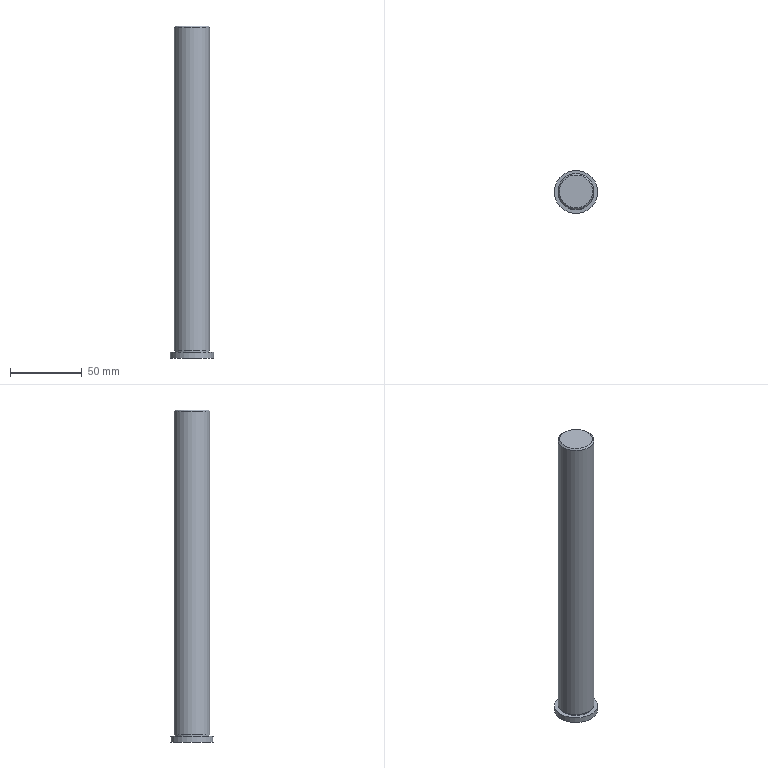Part | STEP file | 1_id634_xmt_txt | 1 solid | 8 faces | box 30 x 30 x 231 mm | volume 114179 mm3 | plane 4 | cylinder 3 | cone 1 | commonest cylinder face diameters 24 x1 25 x1 30 x1
STEP:
#1=CARTESIAN_POINT('',(-84.,-130.,-214.));
#2=VERTEX_POINT('',#1);
#3=CARTESIAN_POINT('',(-99.,-130.,-214.));
#4=DIRECTION('',(0.,0.,-1.));
#5=DIRECTION('',(1.,0.,0.));
#6=AXIS2_PLACEMENT_3D('',#3,#4,#5);
#7=CIRCLE('',#6,15.);
#8=EDGE_CURVE('',#2,#2,#7,.T.);
#9=ORIENTED_EDGE('',*,*,#8,.F.);
#10=EDGE_LOOP('',(#9));
#11=FACE_BOUND('',#10,.T.);
#12=CARTESIAN_POINT('',(-84.,-130.,-210.));
#13=VERTEX_POINT('',#12);
#14=CARTESIAN_POINT('',(-99.,-130.,-210.));
#15=DIRECTION('',(0.,0.,1.));
#16=DIRECTION('',(1.,0.,0.));
#17=AXIS2_PLACEMENT_3D('',#14,#15,#16);
#18=CIRCLE('',#17,15.);
#19=EDGE_CURVE('',#13,#13,#18,.T.);
#20=ORIENTED_EDGE('',*,*,#19,.F.);
#21=EDGE_LOOP('',(#20));
#22=FACE_BOUND('',#21,.T.);
#23=CARTESIAN_POINT('',(-99.,-130.,-212.));
#24=DIRECTION('',(0.,0.,1.));
#25=DIRECTION('',(-1.,0.,0.));
#26=AXIS2_PLACEMENT_3D('',#23,#24,#25);
#27=CYLINDRICAL_SURFACE('',#26,15.);
#28=ADVANCED_FACE('',(#11,#22),#27,.T.);
#29=CARTESIAN_POINT('',(-111.,-130.,-209.));
#30=VERTEX_POINT('',#29);
#31=CARTESIAN_POINT('',(-99.,-130.,-209.));
#32=DIRECTION('',(0.,0.,1.));
#33=DIRECTION('',(-1.,0.,0.));
#34=AXIS2_PLACEMENT_3D('',#31,#32,#33);
#35=CIRCLE('',#34,12.);
#36=EDGE_CURVE('',#30,#30,#35,.T.);
#37=ORIENTED_EDGE('',*,*,#36,.F.);
#38=EDGE_LOOP('',(#37));
#39=FACE_BOUND('',#38,.T.);
#40=CARTESIAN_POINT('',(-111.,-130.,-210.));
#41=VERTEX_POINT('',#40);
#42=CARTESIAN_POINT('',(-99.,-130.,-210.));
#43=DIRECTION('',(0.,0.,1.));
#44=DIRECTION('',(-1.,0.,0.));
#45=AXIS2_PLACEMENT_3D('',#42,#43,#44);
#46=CIRCLE('',#45,12.);
#47=EDGE_CURVE('',#41,#41,#46,.T.);
#48=ORIENTED_EDGE('',*,*,#47,.T.);
#49=EDGE_LOOP('',(#48));
#50=FACE_BOUND('',#49,.T.);
#51=CARTESIAN_POINT('',(-99.,-130.,-209.5));
#52=DIRECTION('',(0.,0.,1.));
#53=DIRECTION('',(1.,0.,0.));
#54=AXIS2_PLACEMENT_3D('',#51,#52,#53);
#55=CYLINDRICAL_SURFACE('',#54,12.);
#56=ADVANCED_FACE('',(#39,#50),#55,.T.);
#57=CARTESIAN_POINT('',(-86.5,-130.,-209.));
#58=VERTEX_POINT('',#57);
#59=CARTESIAN_POINT('',(-99.,-130.,-209.));
#60=DIRECTION('',(0.,0.,1.));
#61=DIRECTION('',(1.,0.,0.));
#62=AXIS2_PLACEMENT_3D('',#59,#60,#61);
#63=CIRCLE('',#62,12.5);
#64=EDGE_CURVE('',#58,#58,#63,.T.);
#65=ORIENTED_EDGE('',*,*,#64,.T.);
#66=EDGE_LOOP('',(#65));
#67=FACE_BOUND('',#66,.T.);
#68=CARTESIAN_POINT('',(-111.5,-130.,16.));
#69=VERTEX_POINT('',#68);
#70=CARTESIAN_POINT('',(-99.,-130.,16.));
#71=DIRECTION('',(0.,0.,1.));
#72=DIRECTION('',(-1.,0.,0.));
#73=AXIS2_PLACEMENT_3D('',#70,#71,#72);
#74=CIRCLE('',#73,12.5);
#75=EDGE_CURVE('',#69,#69,#74,.T.);
#76=ORIENTED_EDGE('',*,*,#75,.F.);
#77=EDGE_LOOP('',(#76));
#78=FACE_BOUND('',#77,.T.);
#79=CARTESIAN_POINT('',(-99.,-130.,-96.5));
#80=DIRECTION('',(0.,0.,1.));
#81=DIRECTION('',(-1.,0.,0.));
#82=AXIS2_PLACEMENT_3D('',#79,#80,#81);
#83=CYLINDRICAL_SURFACE('',#82,12.5);
#84=ADVANCED_FACE('',(#67,#78),#83,.T.);
#85=ORIENTED_EDGE('',*,*,#75,.T.);
#86=EDGE_LOOP('',(#85));
#87=FACE_BOUND('',#86,.T.);
#88=CARTESIAN_POINT('',(-110.5,-130.,17.));
#89=VERTEX_POINT('',#88);
#90=CARTESIAN_POINT('',(-99.,-130.,17.));
#91=DIRECTION('',(0.,0.,-1.));
#92=DIRECTION('',(-1.,0.,0.));
#93=AXIS2_PLACEMENT_3D('',#90,#91,#92);
#94=CIRCLE('',#93,11.5);
#95=EDGE_CURVE('',#89,#89,#94,.T.);
#96=ORIENTED_EDGE('',*,*,#95,.T.);
#97=EDGE_LOOP('',(#96));
#98=FACE_BOUND('',#97,.T.);
#99=CARTESIAN_POINT('',(-99.,-130.,17.));
#100=DIRECTION('',(0.,0.,-1.));
#101=DIRECTION('',(1.,0.,0.));
#102=AXIS2_PLACEMENT_3D('',#99,#100,#101);
#103=CONICAL_SURFACE('',#102,11.5,45.);
#104=ADVANCED_FACE('',(#87,#98),#103,.T.);
#105=ORIENTED_EDGE('',*,*,#95,.F.);
#106=EDGE_LOOP('',(#105));
#107=FACE_OUTER_BOUND('',#106,.T.);
#108=CARTESIAN_POINT('',(-99.,-130.,17.));
#109=DIRECTION('',(0.,0.,1.));
#110=DIRECTION('',(-1.,0.,0.));
#111=AXIS2_PLACEMENT_3D('',#108,#109,#110);
#112=PLANE('',#111);
#113=ADVANCED_FACE('',(#107),#112,.T.);
#114=ORIENTED_EDGE('',*,*,#36,.T.);
#115=EDGE_LOOP('',(#114));
#116=FACE_BOUND('',#115,.T.);
#117=ORIENTED_EDGE('',*,*,#64,.F.);
#118=EDGE_LOOP('',(#117));
#119=FACE_BOUND('',#118,.T.);
#120=CARTESIAN_POINT('',(-111.25,-130.,-209.));
#121=DIRECTION('',(0.,0.,1.));
#122=DIRECTION('',(1.,0.,0.));
#123=AXIS2_PLACEMENT_3D('',#120,#121,#122);
#124=PLANE('',#123);
#125=ADVANCED_FACE('',(#116,#119),#124,.F.);
#126=ORIENTED_EDGE('',*,*,#8,.T.);
#127=EDGE_LOOP('',(#126));
#128=FACE_OUTER_BOUND('',#127,.T.);
#129=CARTESIAN_POINT('',(-99.,-130.,-214.));
#130=DIRECTION('',(0.,0.,-1.));
#131=DIRECTION('',(1.,0.,0.));
#132=AXIS2_PLACEMENT_3D('',#129,#130,#131);
#133=PLANE('',#132);
#134=ADVANCED_FACE('',(#128),#133,.T.);
#135=ORIENTED_EDGE('',*,*,#47,.F.);
#136=EDGE_LOOP('',(#135));
#137=FACE_BOUND('',#136,.T.);
#138=ORIENTED_EDGE('',*,*,#19,.T.);
#139=EDGE_LOOP('',(#138));
#140=FACE_BOUND('',#139,.T.);
#141=CARTESIAN_POINT('',(-99.,-130.,-210.));
#142=DIRECTION('',(0.,0.,1.));
#143=DIRECTION('',(-1.,0.,0.));
#144=AXIS2_PLACEMENT_3D('',#141,#142,#143);
#145=PLANE('',#144);
#146=ADVANCED_FACE('',(#137,#140),#145,.T.);
#147=CLOSED_SHELL('',(#28,#56,#84,#104,#113,#125,#134,#146));
#148=MANIFOLD_SOLID_BREP('',#147);
#149=(LENGTH_UNIT()NAMED_UNIT(*)SI_UNIT(.MILLI.,.METRE.));
#150=UNCERTAINTY_MEASURE_WITH_UNIT(LENGTH_MEASURE(0.00002),#149,'','');
#151=(NAMED_UNIT(*)PLANE_ANGLE_UNIT()SI_UNIT($,.RADIAN.));
#152=PLANE_ANGLE_MEASURE_WITH_UNIT(PLANE_ANGLE_MEASURE(0.01745),#151);
#153=DIMENSIONAL_EXPONENTS(0.,0.,0.,0.,0.,0.,0.);
#154=(CONVERSION_BASED_UNIT('DEGREE',#152)NAMED_UNIT(#153)PLANE_ANGLE_UNIT());
#155=(NAMED_UNIT(*)SI_UNIT($,.STERADIAN.)SOLID_ANGLE_UNIT());
#156=(GEOMETRIC_REPRESENTATION_CONTEXT(3)GLOBAL_UNCERTAINTY_ASSIGNED_CONTEXT((#150))GLOBAL_UNIT_ASSIGNED_CONTEXT((#149,#154,#155))REPRESENTATION_CONTEXT('',''));
#157=ADVANCED_BREP_SHAPE_REPRESENTATION('',(#148),#156);